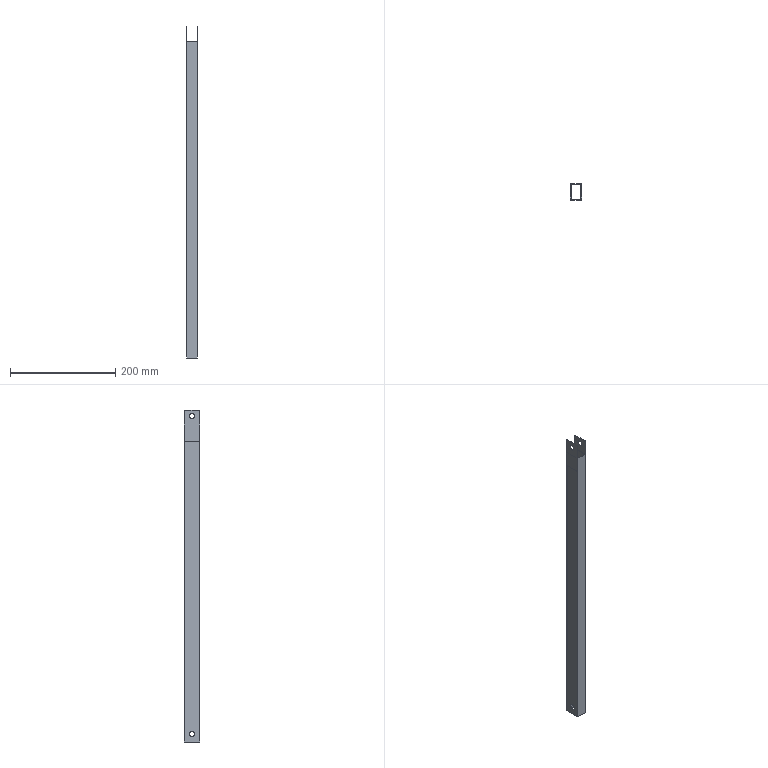Part | SolidWorks | features ICE 3, Extrusion 1, MirrorPattern 1 | 1 solid | 30 faces | box 22 x 30 x 631 mm | volume 60974 mm3 | plane 18 | cylinder 12 | commonest cylinder face diameters 10 x8 6 x4
STEP:
#1=CARTESIAN_POINT('',(1.,-20.,15.));
#2=VERTEX_POINT('',#1);
#3=CARTESIAN_POINT('',(1.,-10.,15.));
#4=VERTEX_POINT('',#3);
#5=CARTESIAN_POINT('',(1.,-15.,15.));
#6=DIRECTION('',(1.,0.,0.));
#7=DIRECTION('',(0.,1.,0.));
#8=AXIS2_PLACEMENT_3D('',#5,#6,#7);
#9=CIRCLE('',#8,5.);
#10=EDGE_CURVE('',#2,#4,#9,.T.);
#11=ORIENTED_EDGE('',*,*,#10,.T.);
#12=CARTESIAN_POINT('',(0.,-10.,15.));
#13=VERTEX_POINT('',#12);
#14=CARTESIAN_POINT('',(21.,-10.,15.));
#15=DIRECTION('',(-1.,0.,0.));
#16=VECTOR('',#15,1000.);
#17=LINE('',#14,#16);
#18=EDGE_CURVE('',#4,#13,#17,.T.);
#19=ORIENTED_EDGE('',*,*,#18,.T.);
#20=CARTESIAN_POINT('',(0.,-20.,15.));
#21=VERTEX_POINT('',#20);
#22=CARTESIAN_POINT('',(0.,-15.,15.));
#23=DIRECTION('',(-1.,0.,0.));
#24=DIRECTION('',(0.,-1.,0.));
#25=AXIS2_PLACEMENT_3D('',#22,#23,#24);
#26=CIRCLE('',#25,5.);
#27=EDGE_CURVE('',#13,#21,#26,.T.);
#28=ORIENTED_EDGE('',*,*,#27,.T.);
#29=CARTESIAN_POINT('',(21.,-20.,15.));
#30=DIRECTION('',(-1.,0.,0.));
#31=VECTOR('',#30,1000.);
#32=LINE('',#29,#31);
#33=EDGE_CURVE('',#2,#21,#32,.T.);
#34=ORIENTED_EDGE('',*,*,#33,.F.);
#35=EDGE_LOOP('',(#11,#19,#28,#34));
#36=FACE_OUTER_BOUND('',#35,.T.);
#37=CARTESIAN_POINT('',(21.,-15.,15.));
#38=DIRECTION('',(-1.,0.,0.));
#39=DIRECTION('',(0.,-1.,0.));
#40=AXIS2_PLACEMENT_3D('',#37,#38,#39);
#41=CYLINDRICAL_SURFACE('',#40,5.);
#42=ADVANCED_FACE('',(#36),#41,.F.);
#43=CARTESIAN_POINT('',(20.,-10.,15.));
#44=VERTEX_POINT('',#43);
#45=CARTESIAN_POINT('',(20.,-20.,15.));
#46=VERTEX_POINT('',#45);
#47=CARTESIAN_POINT('',(20.,-15.,15.));
#48=DIRECTION('',(-1.,0.,0.));
#49=DIRECTION('',(0.,-1.,0.));
#50=AXIS2_PLACEMENT_3D('',#47,#48,#49);
#51=CIRCLE('',#50,5.);
#52=EDGE_CURVE('',#44,#46,#51,.T.);
#53=ORIENTED_EDGE('',*,*,#52,.F.);
#54=CARTESIAN_POINT('',(19.,-10.,15.));
#55=VERTEX_POINT('',#54);
#56=CARTESIAN_POINT('',(21.,-10.,15.));
#57=DIRECTION('',(-1.,0.,0.));
#58=VECTOR('',#57,1000.);
#59=LINE('',#56,#58);
#60=EDGE_CURVE('',#44,#55,#59,.T.);
#61=ORIENTED_EDGE('',*,*,#60,.T.);
#62=CARTESIAN_POINT('',(19.,-20.,15.));
#63=VERTEX_POINT('',#62);
#64=CARTESIAN_POINT('',(19.,-15.,15.));
#65=DIRECTION('',(-1.,0.,0.));
#66=DIRECTION('',(0.,-1.,0.));
#67=AXIS2_PLACEMENT_3D('',#64,#65,#66);
#68=CIRCLE('',#67,5.);
#69=EDGE_CURVE('',#55,#63,#68,.T.);
#70=ORIENTED_EDGE('',*,*,#69,.T.);
#71=CARTESIAN_POINT('',(21.,-20.,15.));
#72=DIRECTION('',(-1.,0.,0.));
#73=VECTOR('',#72,1000.);
#74=LINE('',#71,#73);
#75=EDGE_CURVE('',#46,#63,#74,.T.);
#76=ORIENTED_EDGE('',*,*,#75,.F.);
#77=EDGE_LOOP('',(#53,#61,#70,#76));
#78=FACE_OUTER_BOUND('',#77,.T.);
#79=CARTESIAN_POINT('',(21.,-15.,15.));
#80=DIRECTION('',(-1.,0.,0.));
#81=DIRECTION('',(0.,-1.,0.));
#82=AXIS2_PLACEMENT_3D('',#79,#80,#81);
#83=CYLINDRICAL_SURFACE('',#82,5.);
#84=ADVANCED_FACE('',(#78),#83,.F.);
#85=CARTESIAN_POINT('',(-1.,-20.,619.5));
#86=VERTEX_POINT('',#85);
#87=CARTESIAN_POINT('',(-1.,-10.,619.5));
#88=VERTEX_POINT('',#87);
#89=CARTESIAN_POINT('',(-1.,-15.,619.5));
#90=DIRECTION('',(1.,0.,0.));
#91=DIRECTION('',(0.,1.,0.));
#92=AXIS2_PLACEMENT_3D('',#89,#90,#91);
#93=CIRCLE('',#92,5.);
#94=EDGE_CURVE('',#86,#88,#93,.T.);
#95=ORIENTED_EDGE('',*,*,#94,.F.);
#96=CARTESIAN_POINT('',(0.,-20.,619.5));
#97=VERTEX_POINT('',#96);
#98=CARTESIAN_POINT('',(-1.,-20.,619.5));
#99=DIRECTION('',(1.,0.,0.));
#100=VECTOR('',#99,1000.);
#101=LINE('',#98,#100);
#102=EDGE_CURVE('',#86,#97,#101,.T.);
#103=ORIENTED_EDGE('',*,*,#102,.T.);
#104=CARTESIAN_POINT('',(0.,-10.,619.5));
#105=VERTEX_POINT('',#104);
#106=CARTESIAN_POINT('',(0.,-15.,619.5));
#107=DIRECTION('',(-1.,0.,0.));
#108=DIRECTION('',(0.,-1.,0.));
#109=AXIS2_PLACEMENT_3D('',#106,#107,#108);
#110=CIRCLE('',#109,5.);
#111=EDGE_CURVE('',#105,#97,#110,.T.);
#112=ORIENTED_EDGE('',*,*,#111,.F.);
#113=CARTESIAN_POINT('',(-1.,-10.,619.5));
#114=DIRECTION('',(1.,0.,0.));
#115=VECTOR('',#114,1000.);
#116=LINE('',#113,#115);
#117=EDGE_CURVE('',#88,#105,#116,.T.);
#118=ORIENTED_EDGE('',*,*,#117,.F.);
#119=EDGE_LOOP('',(#95,#103,#112,#118));
#120=FACE_OUTER_BOUND('',#119,.T.);
#121=CARTESIAN_POINT('',(-1.,-15.,619.5));
#122=DIRECTION('',(1.,0.,0.));
#123=DIRECTION('',(0.,1.,0.));
#124=AXIS2_PLACEMENT_3D('',#121,#122,#123);
#125=CYLINDRICAL_SURFACE('',#124,5.);
#126=ADVANCED_FACE('',(#120),#125,.F.);
#127=CARTESIAN_POINT('',(20.,-20.,619.5));
#128=VERTEX_POINT('',#127);
#129=CARTESIAN_POINT('',(20.,-10.,619.5));
#130=VERTEX_POINT('',#129);
#131=CARTESIAN_POINT('',(20.,-15.,619.5));
#132=DIRECTION('',(1.,0.,0.));
#133=DIRECTION('',(0.,1.,0.));
#134=AXIS2_PLACEMENT_3D('',#131,#132,#133);
#135=CIRCLE('',#134,5.);
#136=EDGE_CURVE('',#128,#130,#135,.T.);
#137=ORIENTED_EDGE('',*,*,#136,.F.);
#138=CARTESIAN_POINT('',(21.,-20.,619.5));
#139=VERTEX_POINT('',#138);
#140=CARTESIAN_POINT('',(-1.,-20.,619.5));
#141=DIRECTION('',(1.,0.,0.));
#142=VECTOR('',#141,1000.);
#143=LINE('',#140,#142);
#144=EDGE_CURVE('',#128,#139,#143,.T.);
#145=ORIENTED_EDGE('',*,*,#144,.T.);
#146=CARTESIAN_POINT('',(21.,-10.,619.5));
#147=VERTEX_POINT('',#146);
#148=CARTESIAN_POINT('',(21.,-15.,619.5));
#149=DIRECTION('',(1.,0.,0.));
#150=DIRECTION('',(0.,1.,0.));
#151=AXIS2_PLACEMENT_3D('',#148,#149,#150);
#152=CIRCLE('',#151,5.);
#153=EDGE_CURVE('',#139,#147,#152,.T.);
#154=ORIENTED_EDGE('',*,*,#153,.T.);
#155=CARTESIAN_POINT('',(-1.,-10.,619.5));
#156=DIRECTION('',(1.,0.,0.));
#157=VECTOR('',#156,1000.);
#158=LINE('',#155,#157);
#159=EDGE_CURVE('',#130,#147,#158,.T.);
#160=ORIENTED_EDGE('',*,*,#159,.F.);
#161=EDGE_LOOP('',(#137,#145,#154,#160));
#162=FACE_OUTER_BOUND('',#161,.T.);
#163=CARTESIAN_POINT('',(-1.,-15.,619.5));
#164=DIRECTION('',(1.,0.,0.));
#165=DIRECTION('',(0.,1.,0.));
#166=AXIS2_PLACEMENT_3D('',#163,#164,#165);
#167=CYLINDRICAL_SURFACE('',#166,5.);
#168=ADVANCED_FACE('',(#162),#167,.F.);
#169=CARTESIAN_POINT('',(0.,-15.,15.));
#170=DIRECTION('',(-1.,0.,0.));
#171=DIRECTION('',(0.,-1.,0.));
#172=AXIS2_PLACEMENT_3D('',#169,#170,#171);
#173=CIRCLE('',#172,5.);
#174=EDGE_CURVE('',#21,#13,#173,.T.);
#175=ORIENTED_EDGE('',*,*,#174,.F.);
#176=ORIENTED_EDGE('',*,*,#27,.F.);
#177=EDGE_LOOP('',(#175,#176));
#178=FACE_BOUND('',#177,.T.);
#179=CARTESIAN_POINT('',(0.,0.,571.));
#180=VERTEX_POINT('',#179);
#181=CARTESIAN_POINT('',(0.,-30.,571.));
#182=VERTEX_POINT('',#181);
#183=CARTESIAN_POINT('',(0.,-30.,571.));
#184=DIRECTION('',(0.,-1.,0.));
#185=VECTOR('',#184,1000.);
#186=LINE('',#183,#185);
#187=EDGE_CURVE('',#180,#182,#186,.T.);
#188=ORIENTED_EDGE('',*,*,#187,.F.);
#189=CARTESIAN_POINT('',(0.,0.,0.));
#190=VERTEX_POINT('',#189);
#191=CARTESIAN_POINT('',(0.,0.,601.));
#192=DIRECTION('',(0.,0.,-1.));
#193=VECTOR('',#192,1000.);
#194=LINE('',#191,#193);
#195=EDGE_CURVE('',#180,#190,#194,.T.);
#196=ORIENTED_EDGE('',*,*,#195,.T.);
#197=CARTESIAN_POINT('',(0.,-30.,0.));
#198=VERTEX_POINT('',#197);
#199=CARTESIAN_POINT('',(0.,0.,0.));
#200=DIRECTION('',(0.,-1.,0.));
#201=VECTOR('',#200,1000.);
#202=LINE('',#199,#201);
#203=EDGE_CURVE('',#190,#198,#202,.T.);
#204=ORIENTED_EDGE('',*,*,#203,.T.);
#205=CARTESIAN_POINT('',(0.,-30.,601.));
#206=DIRECTION('',(0.,0.,-1.));
#207=VECTOR('',#206,1000.);
#208=LINE('',#205,#207);
#209=EDGE_CURVE('',#182,#198,#208,.T.);
#210=ORIENTED_EDGE('',*,*,#209,.F.);
#211=EDGE_LOOP('',(#188,#196,#204,#210));
#212=FACE_OUTER_BOUND('',#211,.T.);
#213=CARTESIAN_POINT('',(0.,0.,601.));
#214=DIRECTION('',(1.,0.,0.));
#215=DIRECTION('',(0.,1.,0.));
#216=AXIS2_PLACEMENT_3D('',#213,#214,#215);
#217=PLANE('',#216);
#218=ADVANCED_FACE('',(#178,#212),#217,.F.);
#219=CARTESIAN_POINT('',(0.,0.,601.));
#220=VERTEX_POINT('',#219);
#221=CARTESIAN_POINT('',(0.,-30.,601.));
#222=VERTEX_POINT('',#221);
#223=CARTESIAN_POINT('',(0.,0.,601.));
#224=DIRECTION('',(0.,-1.,0.));
#225=VECTOR('',#224,1000.);
#226=LINE('',#223,#225);
#227=EDGE_CURVE('',#220,#222,#226,.T.);
#228=ORIENTED_EDGE('',*,*,#227,.T.);
#229=CARTESIAN_POINT('',(20.,-30.,601.));
#230=VERTEX_POINT('',#229);
#231=CARTESIAN_POINT('',(0.,-30.,601.));
#232=DIRECTION('',(1.,0.,0.));
#233=VECTOR('',#232,1000.);
#234=LINE('',#231,#233);
#235=EDGE_CURVE('',#222,#230,#234,.T.);
#236=ORIENTED_EDGE('',*,*,#235,.T.);
#237=CARTESIAN_POINT('',(20.,0.,601.));
#238=VERTEX_POINT('',#237);
#239=CARTESIAN_POINT('',(20.,0.,601.));
#240=DIRECTION('',(0.,1.,0.));
#241=VECTOR('',#240,1000.);
#242=LINE('',#239,#241);
#243=EDGE_CURVE('',#230,#238,#242,.T.);
#244=ORIENTED_EDGE('',*,*,#243,.T.);
#245=CARTESIAN_POINT('',(0.,0.,601.));
#246=DIRECTION('',(-1.,0.,0.));
#247=VECTOR('',#246,1000.);
#248=LINE('',#245,#247);
#249=EDGE_CURVE('',#238,#220,#248,.T.);
#250=ORIENTED_EDGE('',*,*,#249,.T.);
#251=EDGE_LOOP('',(#228,#236,#244,#250));
#252=FACE_OUTER_BOUND('',#251,.T.);
#253=CARTESIAN_POINT('',(1.,-29.,601.));
#254=VERTEX_POINT('',#253);
#255=CARTESIAN_POINT('',(19.,-29.,601.));
#256=VERTEX_POINT('',#255);
#257=CARTESIAN_POINT('',(1.,-29.,601.));
#258=DIRECTION('',(1.,0.,0.));
#259=VECTOR('',#258,1000.);
#260=LINE('',#257,#259);
#261=EDGE_CURVE('',#254,#256,#260,.T.);
#262=ORIENTED_EDGE('',*,*,#261,.F.);
#263=CARTESIAN_POINT('',(1.,-1.,601.));
#264=VERTEX_POINT('',#263);
#265=CARTESIAN_POINT('',(1.,-1.,601.));
#266=DIRECTION('',(0.,-1.,0.));
#267=VECTOR('',#266,1000.);
#268=LINE('',#265,#267);
#269=EDGE_CURVE('',#264,#254,#268,.T.);
#270=ORIENTED_EDGE('',*,*,#269,.F.);
#271=CARTESIAN_POINT('',(19.,-1.,601.));
#272=VERTEX_POINT('',#271);
#273=CARTESIAN_POINT('',(1.,-1.,601.));
#274=DIRECTION('',(-1.,0.,0.));
#275=VECTOR('',#274,1000.);
#276=LINE('',#273,#275);
#277=EDGE_CURVE('',#272,#264,#276,.T.);
#278=ORIENTED_EDGE('',*,*,#277,.F.);
#279=CARTESIAN_POINT('',(19.,-1.,601.));
#280=DIRECTION('',(0.,1.,0.));
#281=VECTOR('',#280,1000.);
#282=LINE('',#279,#281);
#283=EDGE_CURVE('',#256,#272,#282,.T.);
#284=ORIENTED_EDGE('',*,*,#283,.F.);
#285=EDGE_LOOP('',(#262,#270,#278,#284));
#286=FACE_BOUND('',#285,.T.);
#287=CARTESIAN_POINT('',(0.,0.,601.));
#288=DIRECTION('',(0.,0.,1.));
#289=DIRECTION('',(1.,0.,0.));
#290=AXIS2_PLACEMENT_3D('',#287,#288,#289);
#291=PLANE('',#290);
#292=ADVANCED_FACE('',(#252,#286),#291,.T.);
#293=ORIENTED_EDGE('',*,*,#203,.F.);
#294=CARTESIAN_POINT('',(20.,0.,0.));
#295=VERTEX_POINT('',#294);
#296=CARTESIAN_POINT('',(0.,0.,0.));
#297=DIRECTION('',(-1.,0.,0.));
#298=VECTOR('',#297,1000.);
#299=LINE('',#296,#298);
#300=EDGE_CURVE('',#295,#190,#299,.T.);
#301=ORIENTED_EDGE('',*,*,#300,.F.);
#302=CARTESIAN_POINT('',(20.,-30.,0.));
#303=VERTEX_POINT('',#302);
#304=CARTESIAN_POINT('',(20.,0.,0.));
#305=DIRECTION('',(0.,1.,0.));
#306=VECTOR('',#305,1000.);
#307=LINE('',#304,#306);
#308=EDGE_CURVE('',#303,#295,#307,.T.);
#309=ORIENTED_EDGE('',*,*,#308,.F.);
#310=CARTESIAN_POINT('',(0.,-30.,0.));
#311=DIRECTION('',(1.,0.,0.));
#312=VECTOR('',#311,1000.);
#313=LINE('',#310,#312);
#314=EDGE_CURVE('',#198,#303,#313,.T.);
#315=ORIENTED_EDGE('',*,*,#314,.F.);
#316=EDGE_LOOP('',(#293,#301,#309,#315));
#317=FACE_OUTER_BOUND('',#316,.T.);
#318=CARTESIAN_POINT('',(1.,-1.,0.));
#319=VERTEX_POINT('',#318);
#320=CARTESIAN_POINT('',(1.,-29.,0.));
#321=VERTEX_POINT('',#320);
#322=CARTESIAN_POINT('',(1.,-1.,0.));
#323=DIRECTION('',(0.,-1.,0.));
#324=VECTOR('',#323,1000.);
#325=LINE('',#322,#324);
#326=EDGE_CURVE('',#319,#321,#325,.T.);
#327=ORIENTED_EDGE('',*,*,#326,.T.);
#328=CARTESIAN_POINT('',(19.,-29.,0.));
#329=VERTEX_POINT('',#328);
#330=CARTESIAN_POINT('',(1.,-29.,0.));
#331=DIRECTION('',(1.,0.,0.));
#332=VECTOR('',#331,1000.);
#333=LINE('',#330,#332);
#334=EDGE_CURVE('',#321,#329,#333,.T.);
#335=ORIENTED_EDGE('',*,*,#334,.T.);
#336=CARTESIAN_POINT('',(19.,-1.,0.));
#337=VERTEX_POINT('',#336);
#338=CARTESIAN_POINT('',(19.,-1.,0.));
#339=DIRECTION('',(0.,1.,0.));
#340=VECTOR('',#339,1000.);
#341=LINE('',#338,#340);
#342=EDGE_CURVE('',#329,#337,#341,.T.);
#343=ORIENTED_EDGE('',*,*,#342,.T.);
#344=CARTESIAN_POINT('',(1.,-1.,0.));
#345=DIRECTION('',(-1.,0.,0.));
#346=VECTOR('',#345,1000.);
#347=LINE('',#344,#346);
#348=EDGE_CURVE('',#337,#319,#347,.T.);
#349=ORIENTED_EDGE('',*,*,#348,.T.);
#350=EDGE_LOOP('',(#327,#335,#343,#349));
#351=FACE_BOUND('',#350,.T.);
#352=CARTESIAN_POINT('',(0.,0.,0.));
#353=DIRECTION('',(0.,0.,1.));
#354=DIRECTION('',(1.,0.,0.));
#355=AXIS2_PLACEMENT_3D('',#352,#353,#354);
#356=PLANE('',#355);
#357=ADVANCED_FACE('',(#317,#351),#356,.F.);
#358=ORIENTED_EDGE('',*,*,#314,.T.);
#359=CARTESIAN_POINT('',(20.,-30.,571.));
#360=VERTEX_POINT('',#359);
#361=CARTESIAN_POINT('',(20.,-30.,601.));
#362=DIRECTION('',(0.,0.,-1.));
#363=VECTOR('',#362,1000.);
#364=LINE('',#361,#363);
#365=EDGE_CURVE('',#360,#303,#364,.T.);
#366=ORIENTED_EDGE('',*,*,#365,.F.);
#367=CARTESIAN_POINT('',(21.,-30.,571.));
#368=VERTEX_POINT('',#367);
#369=CARTESIAN_POINT('',(21.,-30.,571.));
#370=DIRECTION('',(-1.,0.,0.));
#371=VECTOR('',#370,1000.);
#372=LINE('',#369,#371);
#373=EDGE_CURVE('',#368,#360,#372,.T.);
#374=ORIENTED_EDGE('',*,*,#373,.F.);
#375=CARTESIAN_POINT('',(21.,-30.,628.));
#376=VERTEX_POINT('',#375);
#377=CARTESIAN_POINT('',(21.,-30.,601.));
#378=DIRECTION('',(0.,0.,1.));
#379=VECTOR('',#378,1000.);
#380=LINE('',#377,#379);
#381=EDGE_CURVE('',#368,#376,#380,.T.);
#382=ORIENTED_EDGE('',*,*,#381,.T.);
#383=CARTESIAN_POINT('',(20.,-30.,628.));
#384=VERTEX_POINT('',#383);
#385=CARTESIAN_POINT('',(21.,-30.,628.));
#386=DIRECTION('',(-1.,0.,0.));
#387=VECTOR('',#386,1000.);
#388=LINE('',#385,#387);
#389=EDGE_CURVE('',#376,#384,#388,.T.);
#390=ORIENTED_EDGE('',*,*,#389,.T.);
#391=CARTESIAN_POINT('',(20.,-30.,571.));
#392=DIRECTION('',(0.,0.,1.));
#393=VECTOR('',#392,1000.);
#394=LINE('',#391,#393);
#395=EDGE_CURVE('',#230,#384,#394,.T.);
#396=ORIENTED_EDGE('',*,*,#395,.F.);
#397=ORIENTED_EDGE('',*,*,#235,.F.);
#398=CARTESIAN_POINT('',(0.,-30.,628.));
#399=VERTEX_POINT('',#398);
#400=CARTESIAN_POINT('',(0.,-30.,601.));
#401=DIRECTION('',(0.,0.,1.));
#402=VECTOR('',#401,1000.);
#403=LINE('',#400,#402);
#404=EDGE_CURVE('',#222,#399,#403,.T.);
#405=ORIENTED_EDGE('',*,*,#404,.T.);
#406=CARTESIAN_POINT('',(-1.,-30.,628.));
#407=VERTEX_POINT('',#406);
#408=CARTESIAN_POINT('',(-1.,-30.,628.));
#409=DIRECTION('',(1.,0.,0.));
#410=VECTOR('',#409,1000.);
#411=LINE('',#408,#410);
#412=EDGE_CURVE('',#407,#399,#411,.T.);
#413=ORIENTED_EDGE('',*,*,#412,.F.);
#414=CARTESIAN_POINT('',(-1.,-30.,571.));
#415=VERTEX_POINT('',#414);
#416=CARTESIAN_POINT('',(-1.,-30.,571.));
#417=DIRECTION('',(0.,0.,1.));
#418=VECTOR('',#417,1000.);
#419=LINE('',#416,#418);
#420=EDGE_CURVE('',#415,#407,#419,.T.);
#421=ORIENTED_EDGE('',*,*,#420,.F.);
#422=CARTESIAN_POINT('',(-1.,-30.,571.));
#423=DIRECTION('',(1.,0.,0.));
#424=VECTOR('',#423,1000.);
#425=LINE('',#422,#424);
#426=EDGE_CURVE('',#415,#182,#425,.T.);
#427=ORIENTED_EDGE('',*,*,#426,.T.);
#428=ORIENTED_EDGE('',*,*,#209,.T.);
#429=EDGE_LOOP('',(#358,#366,#374,#382,#390,#396,#397,#405,#413,#421,#427,#428));
#430=FACE_OUTER_BOUND('',#429,.T.);
#431=CARTESIAN_POINT('',(0.,-30.,601.));
#432=DIRECTION('',(0.,1.,0.));
#433=DIRECTION('',(0.,0.,1.));
#434=AXIS2_PLACEMENT_3D('',#431,#432,#433);
#435=PLANE('',#434);
#436=ADVANCED_FACE('',(#430),#435,.F.);
#437=CARTESIAN_POINT('',(20.,-15.,15.));
#438=DIRECTION('',(-1.,0.,0.));
#439=DIRECTION('',(0.,-1.,0.));
#440=AXIS2_PLACEMENT_3D('',#437,#438,#439);
#441=CIRCLE('',#440,5.);
#442=EDGE_CURVE('',#46,#44,#441,.T.);
#443=ORIENTED_EDGE('',*,*,#442,.T.);
#444=ORIENTED_EDGE('',*,*,#52,.T.);
#445=EDGE_LOOP('',(#443,#444));
#446=FACE_BOUND('',#445,.T.);
#447=CARTESIAN_POINT('',(20.,0.,571.));
#448=VERTEX_POINT('',#447);
#449=CARTESIAN_POINT('',(20.,0.,601.));
#450=DIRECTION('',(0.,0.,-1.));
#451=VECTOR('',#450,1000.);
#452=LINE('',#449,#451);
#453=EDGE_CURVE('',#448,#295,#452,.T.);
#454=ORIENTED_EDGE('',*,*,#453,.F.);
#455=CARTESIAN_POINT('',(20.,-30.,571.));
#456=DIRECTION('',(0.,-1.,0.));
#457=VECTOR('',#456,1000.);
#458=LINE('',#455,#457);
#459=EDGE_CURVE('',#448,#360,#458,.T.);
#460=ORIENTED_EDGE('',*,*,#459,.T.);
#461=ORIENTED_EDGE('',*,*,#365,.T.);
#462=ORIENTED_EDGE('',*,*,#308,.T.);
#463=EDGE_LOOP('',(#454,#460,#461,#462));
#464=FACE_OUTER_BOUND('',#463,.T.);
#465=CARTESIAN_POINT('',(20.,0.,601.));
#466=DIRECTION('',(-1.,0.,0.));
#467=DIRECTION('',(0.,-1.,0.));
#468=AXIS2_PLACEMENT_3D('',#465,#466,#467);
#469=PLANE('',#468);
#470=ADVANCED_FACE('',(#446,#464),#469,.F.);
#471=ORIENTED_EDGE('',*,*,#300,.T.);
#472=ORIENTED_EDGE('',*,*,#195,.F.);
#473=CARTESIAN_POINT('',(-1.,0.,571.));
#474=VERTEX_POINT('',#473);
#475=CARTESIAN_POINT('',(-1.,0.,571.));
#476=DIRECTION('',(1.,0.,0.));
#477=VECTOR('',#476,1000.);
#478=LINE('',#475,#477);
#479=EDGE_CURVE('',#474,#180,#478,.T.);
#480=ORIENTED_EDGE('',*,*,#479,.F.);
#481=CARTESIAN_POINT('',(-1.,0.,628.));
#482=VERTEX_POINT('',#481);
#483=CARTESIAN_POINT('',(-1.,0.,628.));
#484=DIRECTION('',(0.,0.,-1.));
#485=VECTOR('',#484,1000.);
#486=LINE('',#483,#485);
#487=EDGE_CURVE('',#482,#474,#486,.T.);
#488=ORIENTED_EDGE('',*,*,#487,.F.);
#489=CARTESIAN_POINT('',(0.,0.,628.));
#490=VERTEX_POINT('',#489);
#491=CARTESIAN_POINT('',(-1.,0.,628.));
#492=DIRECTION('',(1.,0.,0.));
#493=VECTOR('',#492,1000.);
#494=LINE('',#491,#493);
#495=EDGE_CURVE('',#482,#490,#494,.T.);
#496=ORIENTED_EDGE('',*,*,#495,.T.);
#497=CARTESIAN_POINT('',(0.,0.,601.));
#498=DIRECTION('',(0.,0.,-1.));
#499=VECTOR('',#498,1000.);
#500=LINE('',#497,#499);
#501=EDGE_CURVE('',#490,#220,#500,.T.);
#502=ORIENTED_EDGE('',*,*,#501,.T.);
#503=ORIENTED_EDGE('',*,*,#249,.F.);
#504=CARTESIAN_POINT('',(20.,0.,628.));
#505=VERTEX_POINT('',#504);
#506=CARTESIAN_POINT('',(20.,0.,628.));
#507=DIRECTION('',(0.,0.,-1.));
#508=VECTOR('',#507,1000.);
#509=LINE('',#506,#508);
#510=EDGE_CURVE('',#505,#238,#509,.T.);
#511=ORIENTED_EDGE('',*,*,#510,.F.);
#512=CARTESIAN_POINT('',(21.,0.,628.));
#513=VERTEX_POINT('',#512);
#514=CARTESIAN_POINT('',(21.,0.,628.));
#515=DIRECTION('',(-1.,0.,0.));
#516=VECTOR('',#515,1000.);
#517=LINE('',#514,#516);
#518=EDGE_CURVE('',#513,#505,#517,.T.);
#519=ORIENTED_EDGE('',*,*,#518,.F.);
#520=CARTESIAN_POINT('',(21.,0.,571.));
#521=VERTEX_POINT('',#520);
#522=CARTESIAN_POINT('',(21.,0.,601.));
#523=DIRECTION('',(0.,0.,-1.));
#524=VECTOR('',#523,1000.);
#525=LINE('',#522,#524);
#526=EDGE_CURVE('',#513,#521,#525,.T.);
#527=ORIENTED_EDGE('',*,*,#526,.T.);
#528=CARTESIAN_POINT('',(21.,0.,571.));
#529=DIRECTION('',(-1.,0.,0.));
#530=VECTOR('',#529,1000.);
#531=LINE('',#528,#530);
#532=EDGE_CURVE('',#521,#448,#531,.T.);
#533=ORIENTED_EDGE('',*,*,#532,.T.);
#534=ORIENTED_EDGE('',*,*,#453,.T.);
#535=EDGE_LOOP('',(#471,#472,#480,#488,#496,#502,#503,#511,#519,#527,#533,#534));
#536=FACE_OUTER_BOUND('',#535,.T.);
#537=CARTESIAN_POINT('',(0.,0.,601.));
#538=DIRECTION('',(0.,-1.,0.));
#539=DIRECTION('',(0.,0.,-1.));
#540=AXIS2_PLACEMENT_3D('',#537,#538,#539);
#541=PLANE('',#540);
#542=ADVANCED_FACE('',(#536),#541,.F.);
#543=ORIENTED_EDGE('',*,*,#10,.F.);
#544=CARTESIAN_POINT('',(1.,-15.,15.));
#545=DIRECTION('',(1.,0.,0.));
#546=DIRECTION('',(0.,1.,0.));
#547=AXIS2_PLACEMENT_3D('',#544,#545,#546);
#548=CIRCLE('',#547,5.);
#549=EDGE_CURVE('',#4,#2,#548,.T.);
#550=ORIENTED_EDGE('',*,*,#549,.F.);
#551=EDGE_LOOP('',(#543,#550));
#552=FACE_BOUND('',#551,.T.);
#553=ORIENTED_EDGE('',*,*,#326,.F.);
#554=CARTESIAN_POINT('',(1.,-1.,601.));
#555=DIRECTION('',(0.,0.,-1.));
#556=VECTOR('',#555,1000.);
#557=LINE('',#554,#556);
#558=EDGE_CURVE('',#264,#319,#557,.T.);
#559=ORIENTED_EDGE('',*,*,#558,.F.);
#560=ORIENTED_EDGE('',*,*,#269,.T.);
#561=CARTESIAN_POINT('',(1.,-29.,601.));
#562=DIRECTION('',(0.,0.,-1.));
#563=VECTOR('',#562,1000.);
#564=LINE('',#561,#563);
#565=EDGE_CURVE('',#254,#321,#564,.T.);
#566=ORIENTED_EDGE('',*,*,#565,.T.);
#567=EDGE_LOOP('',(#553,#559,#560,#566));
#568=FACE_OUTER_BOUND('',#567,.T.);
#569=CARTESIAN_POINT('',(1.,-1.,601.));
#570=DIRECTION('',(1.,0.,0.));
#571=DIRECTION('',(0.,1.,0.));
#572=AXIS2_PLACEMENT_3D('',#569,#570,#571);
#573=PLANE('',#572);
#574=ADVANCED_FACE('',(#552,#568),#573,.T.);
#575=ORIENTED_EDGE('',*,*,#334,.F.);
#576=ORIENTED_EDGE('',*,*,#565,.F.);
#577=ORIENTED_EDGE('',*,*,#261,.T.);
#578=CARTESIAN_POINT('',(19.,-29.,601.));
#579=DIRECTION('',(0.,0.,-1.));
#580=VECTOR('',#579,1000.);
#581=LINE('',#578,#580);
#582=EDGE_CURVE('',#256,#329,#581,.T.);
#583=ORIENTED_EDGE('',*,*,#582,.T.);
#584=EDGE_LOOP('',(#575,#576,#577,#583));
#585=FACE_OUTER_BOUND('',#584,.T.);
#586=CARTESIAN_POINT('',(1.,-29.,601.));
#587=DIRECTION('',(0.,1.,0.));
#588=DIRECTION('',(0.,0.,1.));
#589=AXIS2_PLACEMENT_3D('',#586,#587,#588);
#590=PLANE('',#589);
#591=ADVANCED_FACE('',(#585),#590,.T.);
#592=CARTESIAN_POINT('',(19.,-15.,15.));
#593=DIRECTION('',(-1.,0.,0.));
#594=DIRECTION('',(0.,-1.,0.));
#595=AXIS2_PLACEMENT_3D('',#592,#593,#594);
#596=CIRCLE('',#595,5.);
#597=EDGE_CURVE('',#63,#55,#596,.T.);
#598=ORIENTED_EDGE('',*,*,#597,.F.);
#599=ORIENTED_EDGE('',*,*,#69,.F.);
#600=EDGE_LOOP('',(#598,#599));
#601=FACE_BOUND('',#600,.T.);
#602=ORIENTED_EDGE('',*,*,#342,.F.);
#603=ORIENTED_EDGE('',*,*,#582,.F.);
#604=ORIENTED_EDGE('',*,*,#283,.T.);
#605=CARTESIAN_POINT('',(19.,-1.,601.));
#606=DIRECTION('',(0.,0.,-1.));
#607=VECTOR('',#606,1000.);
#608=LINE('',#605,#607);
#609=EDGE_CURVE('',#272,#337,#608,.T.);
#610=ORIENTED_EDGE('',*,*,#609,.T.);
#611=EDGE_LOOP('',(#602,#603,#604,#610));
#612=FACE_OUTER_BOUND('',#611,.T.);
#613=CARTESIAN_POINT('',(19.,-1.,601.));
#614=DIRECTION('',(-1.,0.,0.));
#615=DIRECTION('',(0.,-1.,0.));
#616=AXIS2_PLACEMENT_3D('',#613,#614,#615);
#617=PLANE('',#616);
#618=ADVANCED_FACE('',(#601,#612),#617,.T.);
#619=ORIENTED_EDGE('',*,*,#348,.F.);
#620=ORIENTED_EDGE('',*,*,#609,.F.);
#621=ORIENTED_EDGE('',*,*,#277,.T.);
#622=ORIENTED_EDGE('',*,*,#558,.T.);
#623=EDGE_LOOP('',(#619,#620,#621,#622));
#624=FACE_OUTER_BOUND('',#623,.T.);
#625=CARTESIAN_POINT('',(1.,-1.,601.));
#626=DIRECTION('',(0.,-1.,0.));
#627=DIRECTION('',(0.,0.,-1.));
#628=AXIS2_PLACEMENT_3D('',#625,#626,#627);
#629=PLANE('',#628);
#630=ADVANCED_FACE('',(#624),#629,.T.);
#631=ORIENTED_EDGE('',*,*,#187,.T.);
#632=ORIENTED_EDGE('',*,*,#426,.F.);
#633=CARTESIAN_POINT('',(-1.,-30.,571.));
#634=DIRECTION('',(0.,-1.,0.));
#635=VECTOR('',#634,1000.);
#636=LINE('',#633,#635);
#637=EDGE_CURVE('',#474,#415,#636,.T.);
#638=ORIENTED_EDGE('',*,*,#637,.F.);
#639=ORIENTED_EDGE('',*,*,#479,.T.);
#640=EDGE_LOOP('',(#631,#632,#638,#639));
#641=FACE_OUTER_BOUND('',#640,.T.);
#642=CARTESIAN_POINT('',(-1.,-30.,571.));
#643=DIRECTION('',(0.,0.,1.));
#644=DIRECTION('',(1.,0.,0.));
#645=AXIS2_PLACEMENT_3D('',#642,#643,#644);
#646=PLANE('',#645);
#647=ADVANCED_FACE('',(#641),#646,.F.);
#648=CARTESIAN_POINT('',(0.,-27.,631.));
#649=VERTEX_POINT('',#648);
#650=CARTESIAN_POINT('',(0.,-27.,628.));
#651=DIRECTION('',(-1.,0.,0.));
#652=DIRECTION('',(0.,1.,0.));
#653=AXIS2_PLACEMENT_3D('',#650,#651,#652);
#654=CIRCLE('',#653,3.);
#655=EDGE_CURVE('',#399,#649,#654,.T.);
#656=ORIENTED_EDGE('',*,*,#655,.T.);
#657=CARTESIAN_POINT('',(-1.,-27.,631.));
#658=VERTEX_POINT('',#657);
#659=CARTESIAN_POINT('',(-1.,-27.,631.));
#660=DIRECTION('',(1.,0.,0.));
#661=VECTOR('',#660,1000.);
#662=LINE('',#659,#661);
#663=EDGE_CURVE('',#658,#649,#662,.T.);
#664=ORIENTED_EDGE('',*,*,#663,.F.);
#665=CARTESIAN_POINT('',(-1.,-27.,628.));
#666=DIRECTION('',(-1.,0.,0.));
#667=DIRECTION('',(0.,1.,0.));
#668=AXIS2_PLACEMENT_3D('',#665,#666,#667);
#669=CIRCLE('',#668,3.);
#670=EDGE_CURVE('',#407,#658,#669,.T.);
#671=ORIENTED_EDGE('',*,*,#670,.F.);
#672=ORIENTED_EDGE('',*,*,#412,.T.);
#673=EDGE_LOOP('',(#656,#664,#671,#672));
#674=FACE_OUTER_BOUND('',#673,.T.);
#675=CARTESIAN_POINT('',(-1.,-27.,628.));
#676=DIRECTION('',(1.,0.,0.));
#677=DIRECTION('',(0.,1.,0.));
#678=AXIS2_PLACEMENT_3D('',#675,#676,#677);
#679=CYLINDRICAL_SURFACE('',#678,3.);
#680=ADVANCED_FACE('',(#674),#679,.T.);
#681=CARTESIAN_POINT('',(0.,-3.,631.));
#682=VERTEX_POINT('',#681);
#683=CARTESIAN_POINT('',(0.,-27.,631.));
#684=DIRECTION('',(0.,1.,0.));
#685=VECTOR('',#684,1000.);
#686=LINE('',#683,#685);
#687=EDGE_CURVE('',#649,#682,#686,.T.);
#688=ORIENTED_EDGE('',*,*,#687,.T.);
#689=CARTESIAN_POINT('',(-1.,-3.,631.));
#690=VERTEX_POINT('',#689);
#691=CARTESIAN_POINT('',(-1.,-3.,631.));
#692=DIRECTION('',(1.,0.,0.));
#693=VECTOR('',#692,1000.);
#694=LINE('',#691,#693);
#695=EDGE_CURVE('',#690,#682,#694,.T.);
#696=ORIENTED_EDGE('',*,*,#695,.F.);
#697=CARTESIAN_POINT('',(-1.,-27.,631.));
#698=DIRECTION('',(0.,1.,0.));
#699=VECTOR('',#698,1000.);
#700=LINE('',#697,#699);
#701=EDGE_CURVE('',#658,#690,#700,.T.);
#702=ORIENTED_EDGE('',*,*,#701,.F.);
#703=ORIENTED_EDGE('',*,*,#663,.T.);
#704=EDGE_LOOP('',(#688,#696,#702,#703));
#705=FACE_OUTER_BOUND('',#704,.T.);
#706=CARTESIAN_POINT('',(-1.,-27.,631.));
#707=DIRECTION('',(0.,0.,-1.));
#708=DIRECTION('',(-1.,0.,0.));
#709=AXIS2_PLACEMENT_3D('',#706,#707,#708);
#710=PLANE('',#709);
#711=ADVANCED_FACE('',(#705),#710,.F.);
#712=CARTESIAN_POINT('',(0.,-3.,628.));
#713=DIRECTION('',(-1.,0.,0.));
#714=DIRECTION('',(0.,-1.,0.));
#715=AXIS2_PLACEMENT_3D('',#712,#713,#714);
#716=CIRCLE('',#715,3.);
#717=EDGE_CURVE('',#682,#490,#716,.T.);
#718=ORIENTED_EDGE('',*,*,#717,.T.);
#719=ORIENTED_EDGE('',*,*,#495,.F.);
#720=CARTESIAN_POINT('',(-1.,-3.,628.));
#721=DIRECTION('',(-1.,0.,0.));
#722=DIRECTION('',(0.,-1.,0.));
#723=AXIS2_PLACEMENT_3D('',#720,#721,#722);
#724=CIRCLE('',#723,3.);
#725=EDGE_CURVE('',#690,#482,#724,.T.);
#726=ORIENTED_EDGE('',*,*,#725,.F.);
#727=ORIENTED_EDGE('',*,*,#695,.T.);
#728=EDGE_LOOP('',(#718,#719,#726,#727));
#729=FACE_OUTER_BOUND('',#728,.T.);
#730=CARTESIAN_POINT('',(-1.,-3.,628.));
#731=DIRECTION('',(1.,0.,0.));
#732=DIRECTION('',(0.,1.,0.));
#733=AXIS2_PLACEMENT_3D('',#730,#731,#732);
#734=CYLINDRICAL_SURFACE('',#733,3.);
#735=ADVANCED_FACE('',(#729),#734,.T.);
#736=CARTESIAN_POINT('',(-1.,-15.,619.5));
#737=DIRECTION('',(1.,0.,0.));
#738=DIRECTION('',(0.,1.,0.));
#739=AXIS2_PLACEMENT_3D('',#736,#737,#738);
#740=CIRCLE('',#739,5.);
#741=EDGE_CURVE('',#88,#86,#740,.T.);
#742=ORIENTED_EDGE('',*,*,#741,.T.);
#743=ORIENTED_EDGE('',*,*,#94,.T.);
#744=EDGE_LOOP('',(#742,#743));
#745=FACE_BOUND('',#744,.T.);
#746=ORIENTED_EDGE('',*,*,#637,.T.);
#747=ORIENTED_EDGE('',*,*,#420,.T.);
#748=ORIENTED_EDGE('',*,*,#670,.T.);
#749=ORIENTED_EDGE('',*,*,#701,.T.);
#750=ORIENTED_EDGE('',*,*,#725,.T.);
#751=ORIENTED_EDGE('',*,*,#487,.T.);
#752=EDGE_LOOP('',(#746,#747,#748,#749,#750,#751));
#753=FACE_OUTER_BOUND('',#752,.T.);
#754=CARTESIAN_POINT('',(-1.,-3.,628.));
#755=DIRECTION('',(-1.,0.,0.));
#756=DIRECTION('',(0.,-1.,0.));
#757=AXIS2_PLACEMENT_3D('',#754,#755,#756);
#758=PLANE('',#757);
#759=ADVANCED_FACE('',(#745,#753),#758,.T.);
#760=ORIENTED_EDGE('',*,*,#111,.T.);
#761=CARTESIAN_POINT('',(0.,-15.,619.5));
#762=DIRECTION('',(-1.,0.,0.));
#763=DIRECTION('',(0.,-1.,0.));
#764=AXIS2_PLACEMENT_3D('',#761,#762,#763);
#765=CIRCLE('',#764,5.);
#766=EDGE_CURVE('',#97,#105,#765,.T.);
#767=ORIENTED_EDGE('',*,*,#766,.T.);
#768=EDGE_LOOP('',(#760,#767));
#769=FACE_BOUND('',#768,.T.);
#770=ORIENTED_EDGE('',*,*,#227,.F.);
#771=ORIENTED_EDGE('',*,*,#501,.F.);
#772=ORIENTED_EDGE('',*,*,#717,.F.);
#773=ORIENTED_EDGE('',*,*,#687,.F.);
#774=ORIENTED_EDGE('',*,*,#655,.F.);
#775=ORIENTED_EDGE('',*,*,#404,.F.);
#776=EDGE_LOOP('',(#770,#771,#772,#773,#774,#775));
#777=FACE_OUTER_BOUND('',#776,.T.);
#778=CARTESIAN_POINT('',(0.,-3.,628.));
#779=DIRECTION('',(-1.,0.,0.));
#780=DIRECTION('',(0.,-1.,0.));
#781=AXIS2_PLACEMENT_3D('',#778,#779,#780);
#782=PLANE('',#781);
#783=ADVANCED_FACE('',(#769,#777),#782,.F.);
#784=ORIENTED_EDGE('',*,*,#459,.F.);
#785=ORIENTED_EDGE('',*,*,#532,.F.);
#786=CARTESIAN_POINT('',(21.,-30.,571.));
#787=DIRECTION('',(0.,-1.,0.));
#788=VECTOR('',#787,1000.);
#789=LINE('',#786,#788);
#790=EDGE_CURVE('',#521,#368,#789,.T.);
#791=ORIENTED_EDGE('',*,*,#790,.T.);
#792=ORIENTED_EDGE('',*,*,#373,.T.);
#793=EDGE_LOOP('',(#784,#785,#791,#792));
#794=FACE_OUTER_BOUND('',#793,.T.);
#795=CARTESIAN_POINT('',(21.,-30.,571.));
#796=DIRECTION('',(0.,0.,-1.));
#797=DIRECTION('',(-1.,0.,0.));
#798=AXIS2_PLACEMENT_3D('',#795,#796,#797);
#799=PLANE('',#798);
#800=ADVANCED_FACE('',(#794),#799,.T.);
#801=CARTESIAN_POINT('',(20.,-3.,631.));
#802=VERTEX_POINT('',#801);
#803=CARTESIAN_POINT('',(20.,-3.,628.));
#804=DIRECTION('',(-1.,0.,0.));
#805=DIRECTION('',(0.,-1.,0.));
#806=AXIS2_PLACEMENT_3D('',#803,#804,#805);
#807=CIRCLE('',#806,3.);
#808=EDGE_CURVE('',#802,#505,#807,.T.);
#809=ORIENTED_EDGE('',*,*,#808,.F.);
#810=CARTESIAN_POINT('',(21.,-3.,631.));
#811=VERTEX_POINT('',#810);
#812=CARTESIAN_POINT('',(21.,-3.,631.));
#813=DIRECTION('',(-1.,0.,0.));
#814=VECTOR('',#813,1000.);
#815=LINE('',#812,#814);
#816=EDGE_CURVE('',#811,#802,#815,.T.);
#817=ORIENTED_EDGE('',*,*,#816,.F.);
#818=CARTESIAN_POINT('',(21.,-3.,628.));
#819=DIRECTION('',(-1.,0.,0.));
#820=DIRECTION('',(0.,-1.,0.));
#821=AXIS2_PLACEMENT_3D('',#818,#819,#820);
#822=CIRCLE('',#821,3.);
#823=EDGE_CURVE('',#811,#513,#822,.T.);
#824=ORIENTED_EDGE('',*,*,#823,.T.);
#825=ORIENTED_EDGE('',*,*,#518,.T.);
#826=EDGE_LOOP('',(#809,#817,#824,#825));
#827=FACE_OUTER_BOUND('',#826,.T.);
#828=CARTESIAN_POINT('',(21.,-3.,628.));
#829=DIRECTION('',(-1.,0.,0.));
#830=DIRECTION('',(0.,-1.,0.));
#831=AXIS2_PLACEMENT_3D('',#828,#829,#830);
#832=CYLINDRICAL_SURFACE('',#831,3.);
#833=ADVANCED_FACE('',(#827),#832,.T.);
#834=CARTESIAN_POINT('',(20.,-27.,631.));
#835=VERTEX_POINT('',#834);
#836=CARTESIAN_POINT('',(20.,-27.,631.));
#837=DIRECTION('',(0.,1.,0.));
#838=VECTOR('',#837,1000.);
#839=LINE('',#836,#838);
#840=EDGE_CURVE('',#835,#802,#839,.T.);
#841=ORIENTED_EDGE('',*,*,#840,.F.);
#842=CARTESIAN_POINT('',(21.,-27.,631.));
#843=VERTEX_POINT('',#842);
#844=CARTESIAN_POINT('',(21.,-27.,631.));
#845=DIRECTION('',(-1.,0.,0.));
#846=VECTOR('',#845,1000.);
#847=LINE('',#844,#846);
#848=EDGE_CURVE('',#843,#835,#847,.T.);
#849=ORIENTED_EDGE('',*,*,#848,.F.);
#850=CARTESIAN_POINT('',(21.,-27.,631.));
#851=DIRECTION('',(0.,1.,0.));
#852=VECTOR('',#851,1000.);
#853=LINE('',#850,#852);
#854=EDGE_CURVE('',#843,#811,#853,.T.);
#855=ORIENTED_EDGE('',*,*,#854,.T.);
#856=ORIENTED_EDGE('',*,*,#816,.T.);
#857=EDGE_LOOP('',(#841,#849,#855,#856));
#858=FACE_OUTER_BOUND('',#857,.T.);
#859=CARTESIAN_POINT('',(21.,-27.,631.));
#860=DIRECTION('',(0.,0.,1.));
#861=DIRECTION('',(1.,0.,0.));
#862=AXIS2_PLACEMENT_3D('',#859,#860,#861);
#863=PLANE('',#862);
#864=ADVANCED_FACE('',(#858),#863,.T.);
#865=CARTESIAN_POINT('',(20.,-27.,628.));
#866=DIRECTION('',(-1.,0.,0.));
#867=DIRECTION('',(0.,1.,0.));
#868=AXIS2_PLACEMENT_3D('',#865,#866,#867);
#869=CIRCLE('',#868,3.);
#870=EDGE_CURVE('',#384,#835,#869,.T.);
#871=ORIENTED_EDGE('',*,*,#870,.F.);
#872=ORIENTED_EDGE('',*,*,#389,.F.);
#873=CARTESIAN_POINT('',(21.,-27.,628.));
#874=DIRECTION('',(-1.,0.,0.));
#875=DIRECTION('',(0.,1.,0.));
#876=AXIS2_PLACEMENT_3D('',#873,#874,#875);
#877=CIRCLE('',#876,3.);
#878=EDGE_CURVE('',#376,#843,#877,.T.);
#879=ORIENTED_EDGE('',*,*,#878,.T.);
#880=ORIENTED_EDGE('',*,*,#848,.T.);
#881=EDGE_LOOP('',(#871,#872,#879,#880));
#882=FACE_OUTER_BOUND('',#881,.T.);
#883=CARTESIAN_POINT('',(21.,-27.,628.));
#884=DIRECTION('',(-1.,0.,0.));
#885=DIRECTION('',(0.,-1.,0.));
#886=AXIS2_PLACEMENT_3D('',#883,#884,#885);
#887=CYLINDRICAL_SURFACE('',#886,3.);
#888=ADVANCED_FACE('',(#882),#887,.T.);
#889=CARTESIAN_POINT('',(21.,-15.,619.5));
#890=DIRECTION('',(1.,0.,0.));
#891=DIRECTION('',(0.,1.,0.));
#892=AXIS2_PLACEMENT_3D('',#889,#890,#891);
#893=CIRCLE('',#892,5.);
#894=EDGE_CURVE('',#147,#139,#893,.T.);
#895=ORIENTED_EDGE('',*,*,#894,.F.);
#896=ORIENTED_EDGE('',*,*,#153,.F.);
#897=EDGE_LOOP('',(#895,#896));
#898=FACE_BOUND('',#897,.T.);
#899=ORIENTED_EDGE('',*,*,#790,.F.);
#900=ORIENTED_EDGE('',*,*,#526,.F.);
#901=ORIENTED_EDGE('',*,*,#823,.F.);
#902=ORIENTED_EDGE('',*,*,#854,.F.);
#903=ORIENTED_EDGE('',*,*,#878,.F.);
#904=ORIENTED_EDGE('',*,*,#381,.F.);
#905=EDGE_LOOP('',(#899,#900,#901,#902,#903,#904));
#906=FACE_OUTER_BOUND('',#905,.T.);
#907=CARTESIAN_POINT('',(21.,-3.,628.));
#908=DIRECTION('',(1.,0.,0.));
#909=DIRECTION('',(0.,-1.,0.));
#910=AXIS2_PLACEMENT_3D('',#907,#908,#909);
#911=PLANE('',#910);
#912=ADVANCED_FACE('',(#898,#906),#911,.T.);
#913=CARTESIAN_POINT('',(20.,-15.,619.5));
#914=DIRECTION('',(1.,0.,0.));
#915=DIRECTION('',(0.,1.,0.));
#916=AXIS2_PLACEMENT_3D('',#913,#914,#915);
#917=CIRCLE('',#916,5.);
#918=EDGE_CURVE('',#130,#128,#917,.T.);
#919=ORIENTED_EDGE('',*,*,#918,.T.);
#920=ORIENTED_EDGE('',*,*,#136,.T.);
#921=EDGE_LOOP('',(#919,#920));
#922=FACE_BOUND('',#921,.T.);
#923=ORIENTED_EDGE('',*,*,#243,.F.);
#924=ORIENTED_EDGE('',*,*,#395,.T.);
#925=ORIENTED_EDGE('',*,*,#870,.T.);
#926=ORIENTED_EDGE('',*,*,#840,.T.);
#927=ORIENTED_EDGE('',*,*,#808,.T.);
#928=ORIENTED_EDGE('',*,*,#510,.T.);
#929=EDGE_LOOP('',(#923,#924,#925,#926,#927,#928));
#930=FACE_OUTER_BOUND('',#929,.T.);
#931=CARTESIAN_POINT('',(20.,-3.,628.));
#932=DIRECTION('',(1.,0.,0.));
#933=DIRECTION('',(0.,-1.,0.));
#934=AXIS2_PLACEMENT_3D('',#931,#932,#933);
#935=PLANE('',#934);
#936=ADVANCED_FACE('',(#922,#930),#935,.F.);
#937=ORIENTED_EDGE('',*,*,#144,.F.);
#938=ORIENTED_EDGE('',*,*,#918,.F.);
#939=ORIENTED_EDGE('',*,*,#159,.T.);
#940=ORIENTED_EDGE('',*,*,#894,.T.);
#941=EDGE_LOOP('',(#937,#938,#939,#940));
#942=FACE_OUTER_BOUND('',#941,.T.);
#943=CARTESIAN_POINT('',(-1.,-15.,619.5));
#944=DIRECTION('',(1.,0.,0.));
#945=DIRECTION('',(0.,1.,0.));
#946=AXIS2_PLACEMENT_3D('',#943,#944,#945);
#947=CYLINDRICAL_SURFACE('',#946,5.);
#948=ADVANCED_FACE('',(#942),#947,.F.);
#949=ORIENTED_EDGE('',*,*,#102,.F.);
#950=ORIENTED_EDGE('',*,*,#741,.F.);
#951=ORIENTED_EDGE('',*,*,#117,.T.);
#952=ORIENTED_EDGE('',*,*,#766,.F.);
#953=EDGE_LOOP('',(#949,#950,#951,#952));
#954=FACE_OUTER_BOUND('',#953,.T.);
#955=CARTESIAN_POINT('',(-1.,-15.,619.5));
#956=DIRECTION('',(1.,0.,0.));
#957=DIRECTION('',(0.,1.,0.));
#958=AXIS2_PLACEMENT_3D('',#955,#956,#957);
#959=CYLINDRICAL_SURFACE('',#958,5.);
#960=ADVANCED_FACE('',(#954),#959,.F.);
#961=ORIENTED_EDGE('',*,*,#60,.F.);
#962=ORIENTED_EDGE('',*,*,#442,.F.);
#963=ORIENTED_EDGE('',*,*,#75,.T.);
#964=ORIENTED_EDGE('',*,*,#597,.T.);
#965=EDGE_LOOP('',(#961,#962,#963,#964));
#966=FACE_OUTER_BOUND('',#965,.T.);
#967=CARTESIAN_POINT('',(21.,-15.,15.));
#968=DIRECTION('',(-1.,0.,0.));
#969=DIRECTION('',(0.,-1.,0.));
#970=AXIS2_PLACEMENT_3D('',#967,#968,#969);
#971=CYLINDRICAL_SURFACE('',#970,5.);
#972=ADVANCED_FACE('',(#966),#971,.F.);
#973=ORIENTED_EDGE('',*,*,#18,.F.);
#974=ORIENTED_EDGE('',*,*,#549,.T.);
#975=ORIENTED_EDGE('',*,*,#33,.T.);
#976=ORIENTED_EDGE('',*,*,#174,.T.);
#977=EDGE_LOOP('',(#973,#974,#975,#976));
#978=FACE_OUTER_BOUND('',#977,.T.);
#979=CARTESIAN_POINT('',(21.,-15.,15.));
#980=DIRECTION('',(-1.,0.,0.));
#981=DIRECTION('',(0.,-1.,0.));
#982=AXIS2_PLACEMENT_3D('',#979,#980,#981);
#983=CYLINDRICAL_SURFACE('',#982,5.);
#984=ADVANCED_FACE('',(#978),#983,.F.);
#985=CLOSED_SHELL('',(#42,#84,#126,#168,#218,#292,#357,#436,#470,#542,#574,#591,#618,#630,#647,#680,#711,#735,#759,#783,#800,#833,#864,#888,#912,#936,#948,#960,#972,#984));
#986=MANIFOLD_SOLID_BREP('',#985);
#987=CARTESIAN_POINT('',(0.,0.,0.));
#988=DIRECTION('',(0.,0.,1.));
#989=DIRECTION('',(1.,0.,0.));
#990=AXIS2_PLACEMENT_3D('',#987,#988,#989);
#991=(LENGTH_UNIT()NAMED_UNIT(*)SI_UNIT(.MILLI.,.METRE.));
#992=UNCERTAINTY_MEASURE_WITH_UNIT(LENGTH_MEASURE(0.00001),#991,'','');
#993=(NAMED_UNIT(*)PLANE_ANGLE_UNIT()SI_UNIT($,.RADIAN.));
#994=(NAMED_UNIT(*)SI_UNIT($,.STERADIAN.)SOLID_ANGLE_UNIT());
#995=(GEOMETRIC_REPRESENTATION_CONTEXT(3)GLOBAL_UNCERTAINTY_ASSIGNED_CONTEXT((#992))GLOBAL_UNIT_ASSIGNED_CONTEXT((#991,#993,#994))REPRESENTATION_CONTEXT('',''));
#996=ADVANCED_BREP_SHAPE_REPRESENTATION('',(#986,#990),#995);